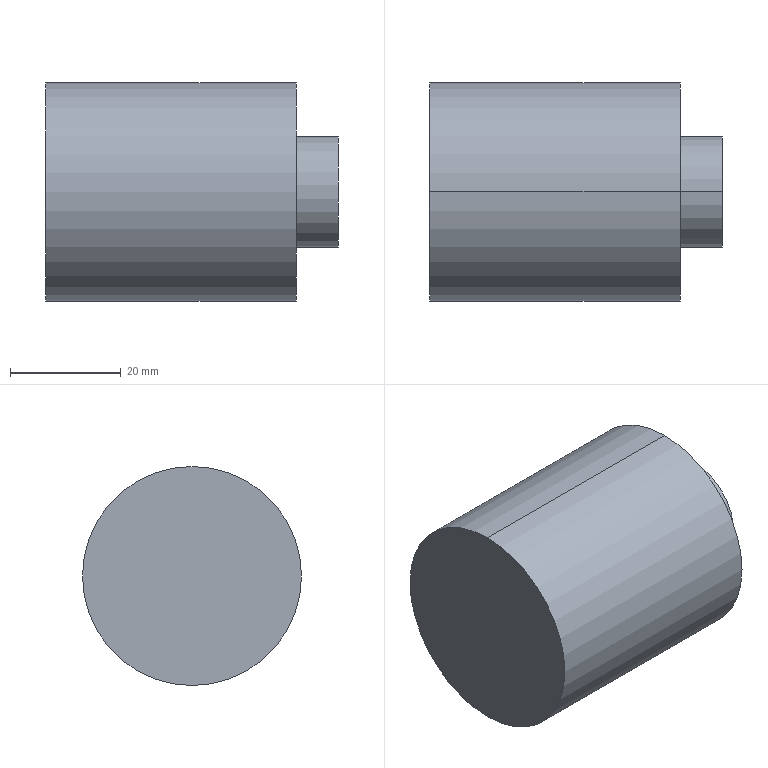Part | SolidWorks | features Extrusion 1, ICE 1 | 1 solid | 7 faces | box 52.8 x 39.5 x 39.5 mm | volume 57776 mm3 | cylinder 4 | plane 3 | commonest cylinder face diameters 20 x2 39.5 x2
STEP:
#1=CARTESIAN_POINT('',(52.8,0.,-10.));
#2=VERTEX_POINT('',#1);
#3=CARTESIAN_POINT('',(52.8,0.,10.));
#4=VERTEX_POINT('',#3);
#5=CARTESIAN_POINT('',(52.8,0.,0.));
#6=DIRECTION('',(1.,0.,0.));
#7=DIRECTION('',(0.,0.,-1.));
#8=AXIS2_PLACEMENT_3D('',#5,#6,#7);
#9=CIRCLE('',#8,10.);
#10=EDGE_CURVE('',#2,#4,#9,.T.);
#11=ORIENTED_EDGE('',*,*,#10,.F.);
#12=CARTESIAN_POINT('',(45.2,0.,-10.));
#13=VERTEX_POINT('',#12);
#14=CARTESIAN_POINT('',(52.8,0.,-10.));
#15=DIRECTION('',(-1.,0.,0.));
#16=VECTOR('',#15,1000.);
#17=LINE('',#14,#16);
#18=EDGE_CURVE('',#2,#13,#17,.T.);
#19=ORIENTED_EDGE('',*,*,#18,.T.);
#20=CARTESIAN_POINT('',(45.2,0.,10.));
#21=VERTEX_POINT('',#20);
#22=CARTESIAN_POINT('',(45.2,0.,0.));
#23=DIRECTION('',(1.,0.,0.));
#24=DIRECTION('',(0.,0.,-1.));
#25=AXIS2_PLACEMENT_3D('',#22,#23,#24);
#26=CIRCLE('',#25,10.);
#27=EDGE_CURVE('',#13,#21,#26,.T.);
#28=ORIENTED_EDGE('',*,*,#27,.T.);
#29=CARTESIAN_POINT('',(52.8,0.,10.));
#30=DIRECTION('',(-1.,0.,0.));
#31=VECTOR('',#30,1000.);
#32=LINE('',#29,#31);
#33=EDGE_CURVE('',#4,#21,#32,.T.);
#34=ORIENTED_EDGE('',*,*,#33,.F.);
#35=EDGE_LOOP('',(#11,#19,#28,#34));
#36=FACE_OUTER_BOUND('',#35,.T.);
#37=CARTESIAN_POINT('',(52.8,0.,0.));
#38=DIRECTION('',(-1.,0.,0.));
#39=DIRECTION('',(0.,0.,1.));
#40=AXIS2_PLACEMENT_3D('',#37,#38,#39);
#41=CYLINDRICAL_SURFACE('',#40,10.);
#42=ADVANCED_FACE('',(#36),#41,.T.);
#43=CARTESIAN_POINT('',(45.2,0.,-19.75));
#44=VERTEX_POINT('',#43);
#45=CARTESIAN_POINT('',(45.2,0.,19.75));
#46=VERTEX_POINT('',#45);
#47=CARTESIAN_POINT('',(45.2,0.,0.));
#48=DIRECTION('',(1.,0.,0.));
#49=DIRECTION('',(0.,0.,-1.));
#50=AXIS2_PLACEMENT_3D('',#47,#48,#49);
#51=CIRCLE('',#50,19.75);
#52=EDGE_CURVE('',#44,#46,#51,.T.);
#53=ORIENTED_EDGE('',*,*,#52,.F.);
#54=CARTESIAN_POINT('',(0.,0.,-19.75));
#55=VERTEX_POINT('',#54);
#56=CARTESIAN_POINT('',(45.2,0.,-19.75));
#57=DIRECTION('',(-1.,0.,0.));
#58=VECTOR('',#57,1000.);
#59=LINE('',#56,#58);
#60=EDGE_CURVE('',#44,#55,#59,.T.);
#61=ORIENTED_EDGE('',*,*,#60,.T.);
#62=CARTESIAN_POINT('',(0.,0.,19.75));
#63=VERTEX_POINT('',#62);
#64=CARTESIAN_POINT('',(0.,0.,0.));
#65=DIRECTION('',(1.,0.,0.));
#66=DIRECTION('',(0.,0.,-1.));
#67=AXIS2_PLACEMENT_3D('',#64,#65,#66);
#68=CIRCLE('',#67,19.75);
#69=EDGE_CURVE('',#55,#63,#68,.T.);
#70=ORIENTED_EDGE('',*,*,#69,.T.);
#71=CARTESIAN_POINT('',(45.2,0.,19.75));
#72=DIRECTION('',(-1.,0.,0.));
#73=VECTOR('',#72,1000.);
#74=LINE('',#71,#73);
#75=EDGE_CURVE('',#46,#63,#74,.T.);
#76=ORIENTED_EDGE('',*,*,#75,.F.);
#77=EDGE_LOOP('',(#53,#61,#70,#76));
#78=FACE_OUTER_BOUND('',#77,.T.);
#79=CARTESIAN_POINT('',(45.2,0.,0.));
#80=DIRECTION('',(-1.,0.,0.));
#81=DIRECTION('',(0.,0.,1.));
#82=AXIS2_PLACEMENT_3D('',#79,#80,#81);
#83=CYLINDRICAL_SURFACE('',#82,19.75);
#84=ADVANCED_FACE('',(#78),#83,.T.);
#85=ORIENTED_EDGE('',*,*,#60,.F.);
#86=CARTESIAN_POINT('',(45.2,0.,0.));
#87=DIRECTION('',(1.,0.,0.));
#88=DIRECTION('',(0.,0.,-1.));
#89=AXIS2_PLACEMENT_3D('',#86,#87,#88);
#90=CIRCLE('',#89,19.75);
#91=EDGE_CURVE('',#46,#44,#90,.T.);
#92=ORIENTED_EDGE('',*,*,#91,.F.);
#93=ORIENTED_EDGE('',*,*,#75,.T.);
#94=CARTESIAN_POINT('',(0.,0.,0.));
#95=DIRECTION('',(1.,0.,0.));
#96=DIRECTION('',(0.,0.,-1.));
#97=AXIS2_PLACEMENT_3D('',#94,#95,#96);
#98=CIRCLE('',#97,19.75);
#99=EDGE_CURVE('',#63,#55,#98,.T.);
#100=ORIENTED_EDGE('',*,*,#99,.T.);
#101=EDGE_LOOP('',(#85,#92,#93,#100));
#102=FACE_OUTER_BOUND('',#101,.T.);
#103=CARTESIAN_POINT('',(45.2,0.,0.));
#104=DIRECTION('',(-1.,0.,0.));
#105=DIRECTION('',(0.,0.,1.));
#106=AXIS2_PLACEMENT_3D('',#103,#104,#105);
#107=CYLINDRICAL_SURFACE('',#106,19.75);
#108=ADVANCED_FACE('',(#102),#107,.T.);
#109=CARTESIAN_POINT('',(45.2,0.,0.));
#110=DIRECTION('',(1.,0.,0.));
#111=DIRECTION('',(0.,0.,-1.));
#112=AXIS2_PLACEMENT_3D('',#109,#110,#111);
#113=CIRCLE('',#112,10.);
#114=EDGE_CURVE('',#21,#13,#113,.T.);
#115=ORIENTED_EDGE('',*,*,#114,.F.);
#116=ORIENTED_EDGE('',*,*,#27,.F.);
#117=EDGE_LOOP('',(#115,#116));
#118=FACE_BOUND('',#117,.T.);
#119=ORIENTED_EDGE('',*,*,#91,.T.);
#120=ORIENTED_EDGE('',*,*,#52,.T.);
#121=EDGE_LOOP('',(#119,#120));
#122=FACE_OUTER_BOUND('',#121,.T.);
#123=CARTESIAN_POINT('',(45.2,0.,0.));
#124=DIRECTION('',(1.,0.,0.));
#125=DIRECTION('',(0.,0.,-1.));
#126=AXIS2_PLACEMENT_3D('',#123,#124,#125);
#127=PLANE('',#126);
#128=ADVANCED_FACE('',(#118,#122),#127,.T.);
#129=ORIENTED_EDGE('',*,*,#99,.F.);
#130=ORIENTED_EDGE('',*,*,#69,.F.);
#131=EDGE_LOOP('',(#129,#130));
#132=FACE_OUTER_BOUND('',#131,.T.);
#133=CARTESIAN_POINT('',(0.,0.,0.));
#134=DIRECTION('',(1.,0.,0.));
#135=DIRECTION('',(0.,0.,-1.));
#136=AXIS2_PLACEMENT_3D('',#133,#134,#135);
#137=PLANE('',#136);
#138=ADVANCED_FACE('',(#132),#137,.F.);
#139=ORIENTED_EDGE('',*,*,#18,.F.);
#140=CARTESIAN_POINT('',(52.8,0.,0.));
#141=DIRECTION('',(1.,0.,0.));
#142=DIRECTION('',(0.,0.,-1.));
#143=AXIS2_PLACEMENT_3D('',#140,#141,#142);
#144=CIRCLE('',#143,10.);
#145=EDGE_CURVE('',#4,#2,#144,.T.);
#146=ORIENTED_EDGE('',*,*,#145,.F.);
#147=ORIENTED_EDGE('',*,*,#33,.T.);
#148=ORIENTED_EDGE('',*,*,#114,.T.);
#149=EDGE_LOOP('',(#139,#146,#147,#148));
#150=FACE_OUTER_BOUND('',#149,.T.);
#151=CARTESIAN_POINT('',(52.8,0.,0.));
#152=DIRECTION('',(-1.,0.,0.));
#153=DIRECTION('',(0.,0.,1.));
#154=AXIS2_PLACEMENT_3D('',#151,#152,#153);
#155=CYLINDRICAL_SURFACE('',#154,10.);
#156=ADVANCED_FACE('',(#150),#155,.T.);
#157=ORIENTED_EDGE('',*,*,#145,.T.);
#158=ORIENTED_EDGE('',*,*,#10,.T.);
#159=EDGE_LOOP('',(#157,#158));
#160=FACE_OUTER_BOUND('',#159,.T.);
#161=CARTESIAN_POINT('',(52.8,0.,0.));
#162=DIRECTION('',(1.,0.,0.));
#163=DIRECTION('',(0.,0.,-1.));
#164=AXIS2_PLACEMENT_3D('',#161,#162,#163);
#165=PLANE('',#164);
#166=ADVANCED_FACE('',(#160),#165,.T.);
#167=CLOSED_SHELL('',(#42,#84,#108,#128,#138,#156,#166));
#168=MANIFOLD_SOLID_BREP('',#167);
#169=CARTESIAN_POINT('',(0.,0.,0.));
#170=DIRECTION('',(0.,0.,1.));
#171=DIRECTION('',(1.,0.,0.));
#172=AXIS2_PLACEMENT_3D('',#169,#170,#171);
#173=(LENGTH_UNIT()NAMED_UNIT(*)SI_UNIT(.MILLI.,.METRE.));
#174=UNCERTAINTY_MEASURE_WITH_UNIT(LENGTH_MEASURE(0.00001),#173,'','');
#175=(NAMED_UNIT(*)PLANE_ANGLE_UNIT()SI_UNIT($,.RADIAN.));
#176=(NAMED_UNIT(*)SI_UNIT($,.STERADIAN.)SOLID_ANGLE_UNIT());
#177=(GEOMETRIC_REPRESENTATION_CONTEXT(3)GLOBAL_UNCERTAINTY_ASSIGNED_CONTEXT((#174))GLOBAL_UNIT_ASSIGNED_CONTEXT((#173,#175,#176))REPRESENTATION_CONTEXT('',''));
#178=ADVANCED_BREP_SHAPE_REPRESENTATION('',(#168,#172),#177);